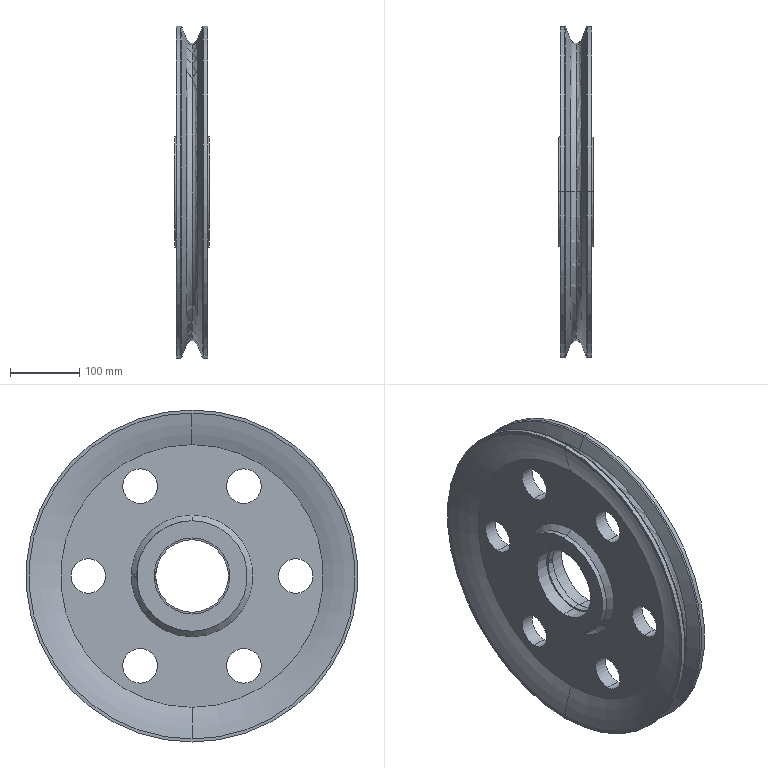Part | SolidWorks | features ICE 2, Chamfer 1, Fillet 1, MirrorPattern 1, RevCut 1, Revolution 1 | 1 solid | 56 faces | box 50 x 480 x 480 mm | volume 3922963 mm3 | cylinder 28 | torus 12 | cone 8 | plane 8 | commonest cylinder face diameters 50 x12 110 x4 160 x4 480 x4 5 x2 105 x2